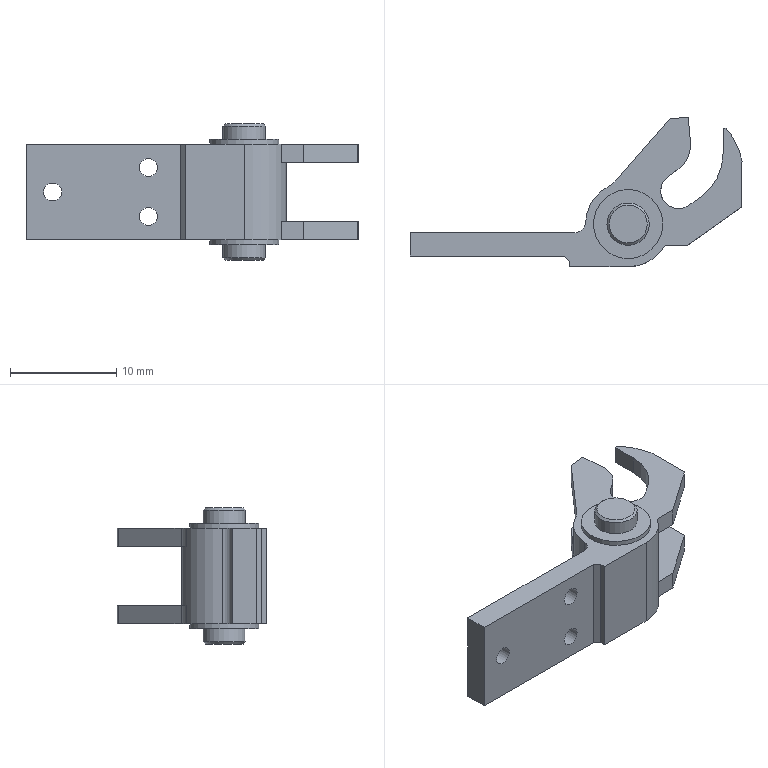CAM job | NX | 3+2 milling | part box 31.196 x 14.046 x 12.8 mm
Tools:
number,name,description,diameter,corner_radius,flute_length,length,flutes
0,C5.0,COUNTERSINKING_TOOL,5.0,0.0,50.0,100.0,2
0,D10-ROUGH-LOWSPEED,MILL,10.0,0.0,50.0,75.0,3
0,D5-ROUGH-LOWSPEED,MILL,5.0,0.0,50.0,75.0,3
0,D3-ROUGH-LOWSPEED,MILL,3.0,0.0,50.0,75.0,3
Operations:
program,operation,operation_type,tool,method,geometry_group,spindle_rpm,surface_speed,feed_per_tooth,feed_cut,feed_plunge,cut_length_mm,path_length_mm,cut_time_min,machine_time_min
OP1,CAVITY_MILL,CavityMilling,D10-ROUGH-LOWSPEED,METHOD,WORKPIECE-1,4500.0,141.372,0.0593,800.0,100.0,1564.314,2166.073,1.955,2.016
OP1,CAVITY_MILL_COPY,CavityMilling,D10-ROUGH-LOWSPEED,METHOD,WORKPIECE-1,4500.0,141.372,0.0741,1000.0,100.0,261.858,360.453,0.2619,0.2717
OP1,FLOOR_WALL,VolumeBased25DMillingOperation,D10-ROUGH-LOWSPEED,METHOD,WORKPIECE-1,4500.0,141.372,0.0593,800.0,100.0,139.074,219.02,0.1738,0.1818
OP1,PLANAR_PROFILE,PlanarMilling,D3-ROUGH-LOWSPEED,METHOD,WORKPIECE-1,15000.0,141.0,0.0178,800.0,100.0,152.07,324.471,0.1901,0.2073
OP2,CAVITY_MILL_COPY_1,CavityMilling,D10-ROUGH-LOWSPEED,METHOD,WORKPIECE-2,4500.0,141.372,0.0593,800.0,100.0,320.679,526.184,0.4008,0.4214
OP2,FLOOR_WALL_COPY,VolumeBased25DMillingOperation,C5.0,METHOD,WORKPIECE-2,5000.0,78.54,0.1,1000.0,100.0,143.821,216.023,0.1438,0.151
OP2,PLANAR_PROFILE_COPY,PlanarMilling,D3-ROUGH-LOWSPEED,METHOD,WORKPIECE-2,6000.0,56.549,0.0222,800.0,100.0,121.035,248.148,0.1513,0.164
OP3,CAVITY_MILL_1,CavityMilling,D5-ROUGH-LOWSPEED,METHOD,WORKPIECE-3,15000.0,235.0,0.0222,1000.0,100.0,2017.513,2221.243,2.018,2.038